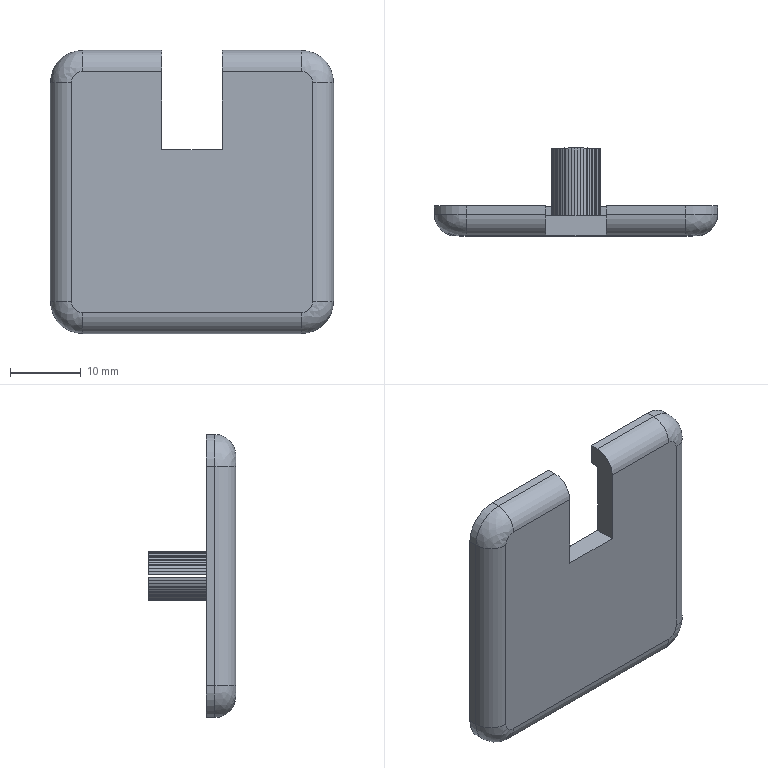Part | STEP file | 1 solid | 133 faces | box 40 x 12.4 x 40 mm | volume 4676 mm3 | plane 66 | cylinder 63 | other 4 | commonest cylinder face diameters 6.6 x24 7 x23 9 x8 6 x5 4.9 x3